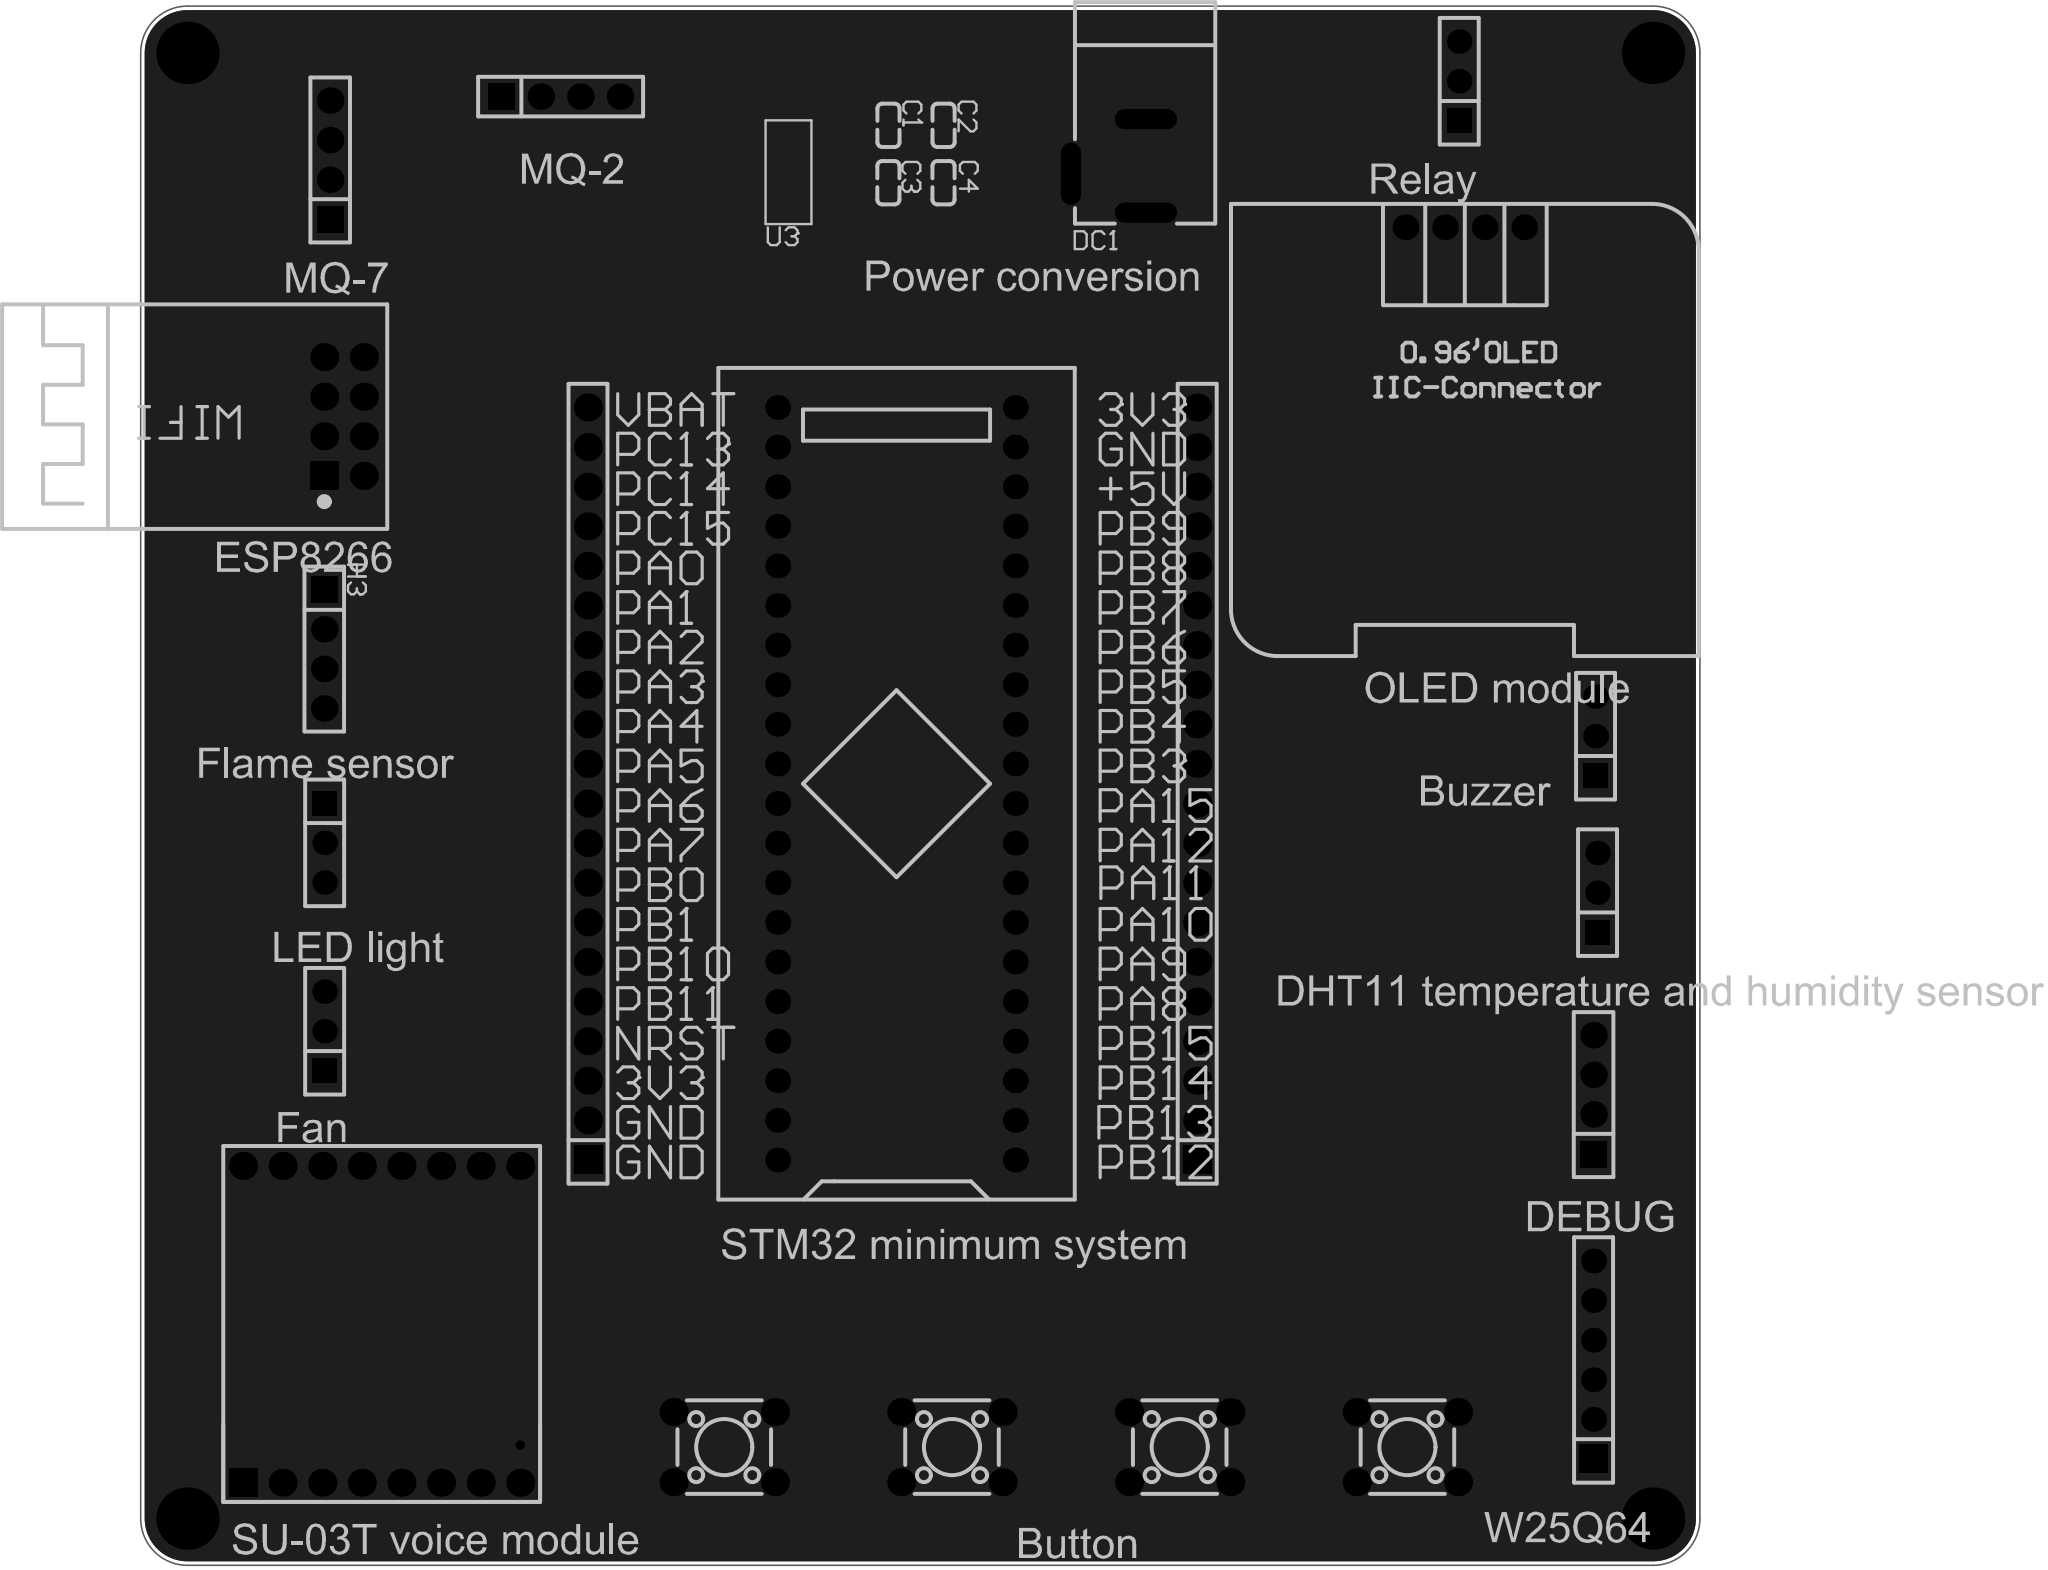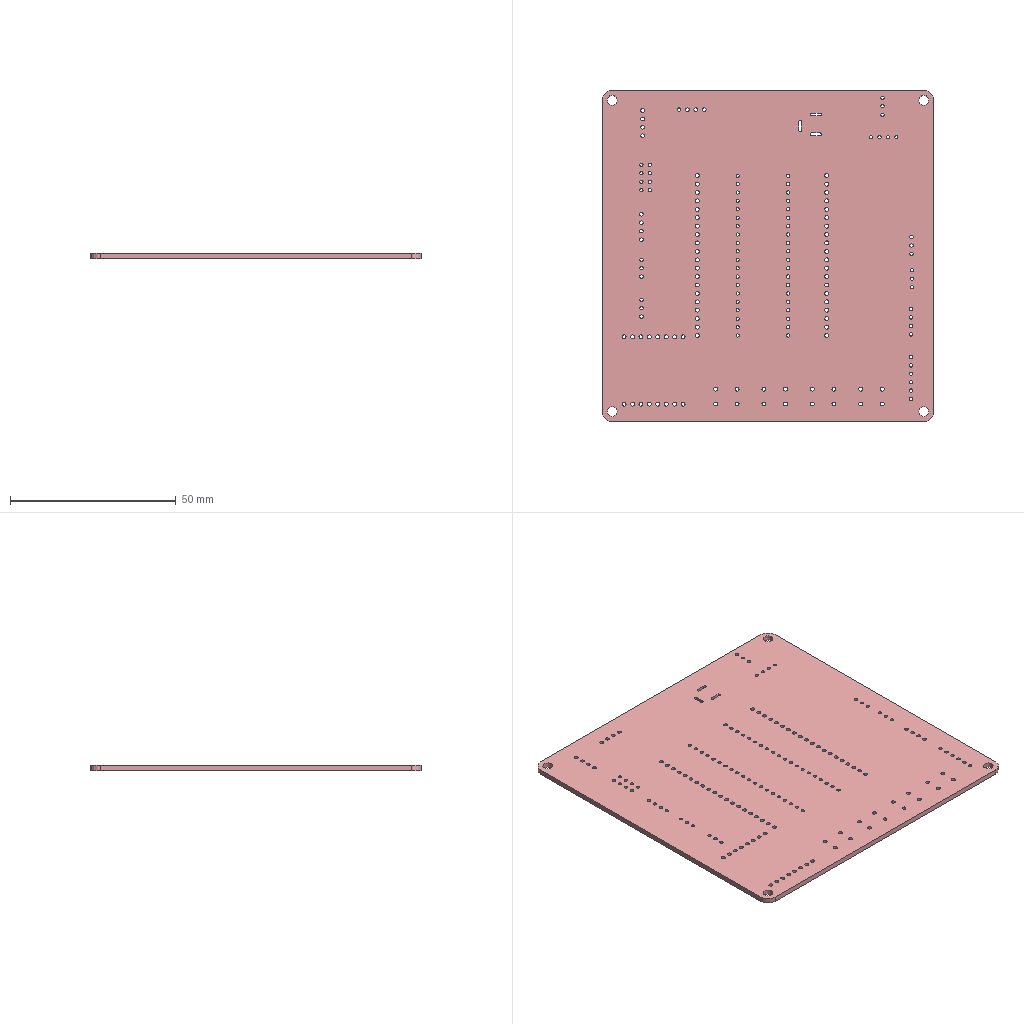Circuit board layout | Altium Designer | box 100 x 100 x 1.6 mm
Layer stack:
# Altium Designer layer stack of  (unit mm; dielectric type: 0 none, 1 core, 2 prepreg, 3 surface material)
index,name,kind,layer,copper_thickness_mm,dielectric_type,dielectric_thickness_mm,dielectric_material,dielectric_constant
0,Top Paste Mask Layer,other,,,,,,
1,Top Silkscreen Layer,other,,,,,,
2,Top Solder Mask Layer,dielectric,,,3,0.01,,3.3
3,Top Layer,copper,Top Layer,0.035,,,,
4,Dielectric1,dielectric,,,3,1.51,FR4,4.5
5,Bottom Layer,copper,Bottom Layer,0.035,,,,
6,Bottom Solder Mask Layer,dielectric,,,3,0.01,,3.3
7,Bottom Silkscreen Layer,other,,,,,,
8,Bottom Paste Mask Layer,other,,,,,,
# drill layer pairs: low layer,high layer
drill_pair,Top Layer,Bottom Layer
Part placement:
Designator,Comment,Layer,Footprint,Center-X(mm),Center-Y(mm),Rotation
U1,STM32F103C8T6-Card,TopLayer,CONN-TH_L53.3-W22.9_STM32F103C8T6-CARD,133.623,129.032,90
H1,,TopLayer,HDR-TH_20P-P2.54-V-F,152.906,129.032,90
H2,,TopLayer,HDR-TH_20P-P2.54-V-F,113.835,129.032,90
OLED1,,TopLayer,0.96OLED_4P,170.072,164.719,0
SW5,,TopLayer,SW-TH_4P-L6.0-W6.0-P4.50-LS6.5,166.389,86.487,0
SW6,,TopLayer,SW-TH_4P-L6.0-W6.0-P4.50-LS6.5,137.179,86.487,0
SW7,,TopLayer,SW-TH_4P-L6.0-W6.0-P4.50-LS6.5,122.574,86.487,0
U2,Ai-Thinker ESP-01S ESP8266,TopLayer,WIFIM-TH_8P-L24.7-W14.4-P2.54,98.19,152.585,180
H7,,TopLayer,HDR-TH_4P-P2.54-V-F,97.301,169.037,90
H10,,TopLayer,HDR-TH_3P-P2.54-V-F,96.945,125.24,270
H11,,TopLayer,HDR-TH_3P-P2.54-V-F,96.945,113.157,90
H12,,TopLayer,HDR-TH_3P-P2.54-V-F,169.71,174.088,90
H13,,TopLayer,HDR-TH_3P-P2.54-V-F,178.581,122.047,90
H14,,TopLayer,HDR-TH_6P-P2.54-V-F,178.327,92.075,90
H6,,TopLayer,HDR-TH_4P-P2.54-V-F,112.078,173.101,0
H8,,TopLayer,HDR-TH_4P-P2.54-V-F,178.327,109.093,90
H9,,TopLayer,HDR-TH_16P-P2.54-V-M-R2-C8-S2.54,100.603,94.361,0
SW1,,TopLayer,SW-TH_4P-L6.0-W6.0-P4.50-LS6.5,151.784,86.487,0
C1,100nF,TopLayer,C0603,133.105,171.26,270
C2,100nF,TopLayer,C0603,136.639,171.26,270
C3,100nF,TopLayer,C0603,133.101,167.577,90
C4,100nF,TopLayer,C0603,136.635,167.577,90
U3,AMS1117-3.3,TopLayer,SOT-223-3_L6.5-W3.4-P2.30-LS7.0-BR,126.794,168.252,0
DC1,,TopLayer,DC-2.0,147.212,168.656,90
H3,,TopLayer,HDR-TH_4P-P2.54-V-F,96.92,137.668,270
H4,,TopLayer,HDR-TH_3P-P2.54-V-F,178.454,132.08,90
Pad and via stacks:
# Altium Designer via and pad stacks of  (unit mm). Each distinct definition once, with the count of objects using it.
# via: kind,start_layer,end_layer,hole_mm,diameter_mm,mode(0 simple;1 top-mid-bottom;2 full stack),diameter_per_layer,count,example_net
# pad: kind,layer,hole_mm,hole_type(0 round;1 square;2 slot),plating,top_size,top_shape(1 round;2 rect;3 octagon;9 rounded rect),mid_size,bottom_size,mode,footprint,size_per_layer,count,example
pad,Multi-Layer,3,0,plated,4x4,1,4x4,4x4,0,,,4,1
pad,Multi-Layer,1,0,plated,1.6x1.6,1,1.6x1.6,1.6x1.6,0,CONN-TH_L53.3-W22.9_STM32F103C8T6-CARD,,40,U1.1
pad,Multi-Layer,1.2,0,plated,1.8x1.8,2,1.8x1.8,1.8x1.8,0,HDR-TH_20P-P2.54-V-F,,2,H1.1
pad,Multi-Layer,1.2,0,plated,1.8x1.8,1,1.8x1.8,1.8x1.8,0,HDR-TH_20P-P2.54-V-F,,38,H1.2
pad,Multi-Layer,1,0,plated,1.65x1.65,1,1.65x1.65,1.65x1.65,0,0.96OLED_4P,,4,OLED1.4
pad,Multi-Layer,1.2,0,plated,1.8x1.8,1,1.8x1.8,1.8x1.8,0,SW-TH_4P-L6.0-W6.0-P4.50-LS6.5,,16,SW5.1
pad,Multi-Layer,1,0,plated,1.8x1.8,1,1.8x1.8,1.8x1.8,0,WIFIM-TH_8P-L24.7-W14.4-P2.54,,7,U2.8
pad,Multi-Layer,1,0,plated,1.8x1.8,2,1.8x1.8,1.8x1.8,0,WIFIM-TH_8P-L24.7-W14.4-P2.54,,1,U2.1
pad,Multi-Layer,1.1,0,plated,1.7x1.7,2,1.7x1.7,1.7x1.7,0,HDR-TH_4P-P2.54-V-F,,4,H7.1
pad,Multi-Layer,1.1,0,plated,1.7x1.7,1,1.7x1.7,1.7x1.7,0,HDR-TH_4P-P2.54-V-F,,12,H7.2
pad,Multi-Layer,1.02,0,plated,1.575x1.575,1,1.575x1.575,1.575x1.575,0,HDR-TH_3P-P2.54-V-F,,10,H10.3
pad,Multi-Layer,1.02,0,plated,1.575x1.575,2,1.575x1.575,1.575x1.575,0,HDR-TH_3P-P2.54-V-F,,5,H10.1
pad,Multi-Layer,1.02,0,plated,1.6x1.6,1,1.6x1.6,1.6x1.6,0,HDR-TH_6P-P2.54-V-F,,5,H14.6
pad,Multi-Layer,1.02,0,plated,1.8x1.8,2,1.8x1.8,1.8x1.8,0,HDR-TH_6P-P2.54-V-F,,1,H14.1
pad,Multi-Layer,1.2,0,plated,1.8x1.8,1,1.8x1.8,1.8x1.8,0,HDR-TH_16P-P2.54-V-M-R2-C8-S2.54,,15,H9.16
pad,Multi-Layer,1.2,0,plated,1.8x1.8,2,1.8x1.8,1.8x1.8,0,HDR-TH_16P-P2.54-V-M-R2-C8-S2.54,,1,H9.1
pad,Multi-Layer,0.8001,2,plated,4x1.3,1,4x1.3,4x1.3,0,DC-2.0,,3,DC1.2
pad,Top Layer,0,0,plated,0.8x0.9,2,0.8x0.9,0.8x0.9,0,C0603,,8,C1.2
pad,Top Layer,0,0,plated,2.5x1.1,2,2.5x1.1,2.5x1.1,0,SOT-223-3_L6.5-W3.4-P2.30-LS7.0-BR,,3,U3.1
pad,Top Layer,0,0,plated,2.34x3.6,2,2.34x3.6,2.34x3.6,0,SOT-223-3_L6.5-W3.4-P2.30-LS7.0-BR,,1,U3.4
via,Top Layer,Bottom Layer,0.3048,0.61,0,,1,GND
Copper pours:
name,layer,net,type(0 solid;1 hatched;2 none)
Bottom Layer-GND,Bottom Layer,GND,0
Top Layer-GND,Top Layer,GND,0